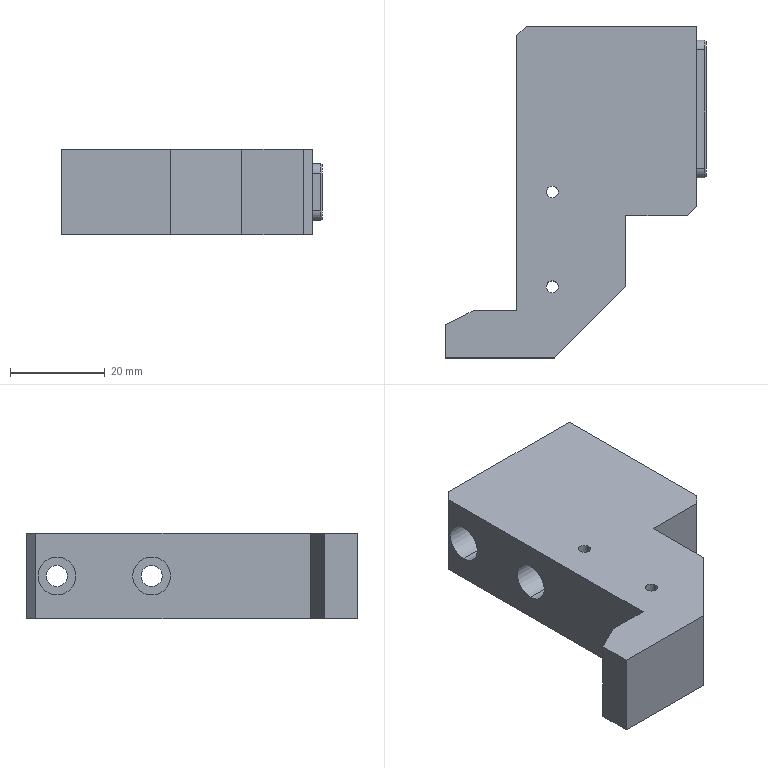Part | NX | features BREP 1 | 1 solid | 45 faces | box 55 x 70 x 18 mm | volume 37396 mm3 | plane 25 | cylinder 16 | cone 4 | commonest cylinder face diameters 2.5 x4 4 x4 4.5 x4 8 x4
STEP:
#1=CARTESIAN_POINT('',(-36.,70.,9.));
#2=VERTEX_POINT('',#1);
#3=CARTESIAN_POINT('',(-38.,68.,9.));
#4=VERTEX_POINT('',#3);
#5=CARTESIAN_POINT('',(-53.,53.,9.));
#6=DIRECTION('',(-0.7071,-0.7071,0.));
#7=VECTOR('',#6,1000.);
#8=LINE('',#5,#7);
#9=EDGE_CURVE('',#2,#4,#8,.T.);
#10=ORIENTED_EDGE('',*,*,#9,.F.);
#11=CARTESIAN_POINT('',(-36.,70.,-9.));
#12=VERTEX_POINT('',#11);
#13=CARTESIAN_POINT('',(-36.,70.,9.));
#14=DIRECTION('',(0.,0.,1.));
#15=VECTOR('',#14,1000.);
#16=LINE('',#13,#15);
#17=EDGE_CURVE('',#12,#2,#16,.T.);
#18=ORIENTED_EDGE('',*,*,#17,.F.);
#19=CARTESIAN_POINT('',(-38.,68.,-9.));
#20=VERTEX_POINT('',#19);
#21=CARTESIAN_POINT('',(-38.,68.,-9.));
#22=DIRECTION('',(0.7071,0.7071,0.));
#23=VECTOR('',#22,1000.);
#24=LINE('',#21,#23);
#25=EDGE_CURVE('',#20,#12,#24,.T.);
#26=ORIENTED_EDGE('',*,*,#25,.F.);
#27=CARTESIAN_POINT('',(-38.,68.,9.));
#28=DIRECTION('',(0.,0.,-1.));
#29=VECTOR('',#28,1000.);
#30=LINE('',#27,#29);
#31=EDGE_CURVE('',#4,#20,#30,.T.);
#32=ORIENTED_EDGE('',*,*,#31,.F.);
#33=EDGE_LOOP('',(#10,#18,#26,#32));
#34=FACE_BOUND('',#33,.T.);
#35=CARTESIAN_POINT('',(-38.,68.,9.));
#36=DIRECTION('',(0.7071,-0.7071,0.));
#37=DIRECTION('',(0.,0.,-1.));
#38=AXIS2_PLACEMENT_3D('',#35,#36,#37);
#39=PLANE('',#38);
#40=ADVANCED_FACE('',(#34),#39,.F.);
#41=CARTESIAN_POINT('',(0.,32.,-9.));
#42=VERTEX_POINT('',#41);
#43=CARTESIAN_POINT('',(-2.,30.,-9.));
#44=VERTEX_POINT('',#43);
#45=CARTESIAN_POINT('',(-2.,30.,-9.));
#46=DIRECTION('',(-0.7071,-0.7071,0.));
#47=VECTOR('',#46,1000.);
#48=LINE('',#45,#47);
#49=EDGE_CURVE('',#42,#44,#48,.T.);
#50=ORIENTED_EDGE('',*,*,#49,.F.);
#51=CARTESIAN_POINT('',(0.,32.,9.));
#52=VERTEX_POINT('',#51);
#53=CARTESIAN_POINT('',(0.,32.,9.));
#54=DIRECTION('',(0.,0.,-1.));
#55=VECTOR('',#54,1000.);
#56=LINE('',#53,#55);
#57=EDGE_CURVE('',#52,#42,#56,.T.);
#58=ORIENTED_EDGE('',*,*,#57,.F.);
#59=CARTESIAN_POINT('',(-2.,30.,9.));
#60=VERTEX_POINT('',#59);
#61=CARTESIAN_POINT('',(-16.,16.,9.));
#62=DIRECTION('',(0.7071,0.7071,0.));
#63=VECTOR('',#62,1000.);
#64=LINE('',#61,#63);
#65=EDGE_CURVE('',#60,#52,#64,.T.);
#66=ORIENTED_EDGE('',*,*,#65,.F.);
#67=CARTESIAN_POINT('',(-2.,30.,-9.));
#68=DIRECTION('',(0.,0.,1.));
#69=VECTOR('',#68,1000.);
#70=LINE('',#67,#69);
#71=EDGE_CURVE('',#44,#60,#70,.T.);
#72=ORIENTED_EDGE('',*,*,#71,.F.);
#73=EDGE_LOOP('',(#50,#58,#66,#72));
#74=FACE_BOUND('',#73,.T.);
#75=CARTESIAN_POINT('',(-2.,30.,-9.));
#76=DIRECTION('',(-0.7071,0.7071,0.));
#77=DIRECTION('',(0.,0.,1.));
#78=AXIS2_PLACEMENT_3D('',#75,#76,#77);
#79=PLANE('',#78);
#80=ADVANCED_FACE('',(#74),#79,.F.);
#81=CARTESIAN_POINT('',(-31.75,35.,9.));
#82=VERTEX_POINT('',#81);
#83=CARTESIAN_POINT('',(-31.75,35.,-9.));
#84=VERTEX_POINT('',#83);
#85=CARTESIAN_POINT('',(-31.75,35.,9.));
#86=DIRECTION('',(0.,0.,1.));
#87=VECTOR('',#86,1000.);
#88=LINE('',#85,#87);
#89=EDGE_CURVE('',#82,#84,#88,.F.);
#90=ORIENTED_EDGE('',*,*,#89,.T.);
#91=CARTESIAN_POINT('',(-29.25,35.,-9.));
#92=VERTEX_POINT('',#91);
#93=CARTESIAN_POINT('',(-30.5,35.,-9.));
#94=DIRECTION('',(0.,0.,1.));
#95=DIRECTION('',(1.,0.,0.));
#96=AXIS2_PLACEMENT_3D('',#93,#94,#95);
#97=CIRCLE('',#96,1.25);
#98=EDGE_CURVE('',#92,#84,#97,.T.);
#99=ORIENTED_EDGE('',*,*,#98,.F.);
#100=CARTESIAN_POINT('',(-29.25,35.,9.));
#101=VERTEX_POINT('',#100);
#102=CARTESIAN_POINT('',(-29.25,35.,9.));
#103=DIRECTION('',(0.,0.,1.));
#104=VECTOR('',#103,1000.);
#105=LINE('',#102,#104);
#106=EDGE_CURVE('',#101,#92,#105,.F.);
#107=ORIENTED_EDGE('',*,*,#106,.F.);
#108=CARTESIAN_POINT('',(-30.5,35.,9.));
#109=DIRECTION('',(0.,0.,1.));
#110=DIRECTION('',(1.,0.,0.));
#111=AXIS2_PLACEMENT_3D('',#108,#109,#110);
#112=CIRCLE('',#111,1.25);
#113=EDGE_CURVE('',#101,#82,#112,.T.);
#114=ORIENTED_EDGE('',*,*,#113,.T.);
#115=EDGE_LOOP('',(#90,#99,#107,#114));
#116=FACE_BOUND('',#115,.T.);
#117=CARTESIAN_POINT('',(-30.5,35.,9.));
#118=DIRECTION('',(0.,0.,1.));
#119=DIRECTION('',(1.,0.,0.));
#120=AXIS2_PLACEMENT_3D('',#117,#118,#119);
#121=CYLINDRICAL_SURFACE('',#120,1.25);
#122=ADVANCED_FACE('',(#116),#121,.F.);
#123=CARTESIAN_POINT('',(-31.75,15.,9.));
#124=VERTEX_POINT('',#123);
#125=CARTESIAN_POINT('',(-31.75,15.,-9.));
#126=VERTEX_POINT('',#125);
#127=CARTESIAN_POINT('',(-31.75,15.,9.));
#128=DIRECTION('',(0.,0.,1.));
#129=VECTOR('',#128,1000.);
#130=LINE('',#127,#129);
#131=EDGE_CURVE('',#124,#126,#130,.F.);
#132=ORIENTED_EDGE('',*,*,#131,.T.);
#133=CARTESIAN_POINT('',(-29.25,15.,-9.));
#134=VERTEX_POINT('',#133);
#135=CARTESIAN_POINT('',(-30.5,15.,-9.));
#136=DIRECTION('',(0.,0.,1.));
#137=DIRECTION('',(1.,0.,0.));
#138=AXIS2_PLACEMENT_3D('',#135,#136,#137);
#139=CIRCLE('',#138,1.25);
#140=EDGE_CURVE('',#134,#126,#139,.T.);
#141=ORIENTED_EDGE('',*,*,#140,.F.);
#142=CARTESIAN_POINT('',(-29.25,15.,9.));
#143=VERTEX_POINT('',#142);
#144=CARTESIAN_POINT('',(-29.25,15.,9.));
#145=DIRECTION('',(0.,0.,1.));
#146=VECTOR('',#145,1000.);
#147=LINE('',#144,#146);
#148=EDGE_CURVE('',#143,#134,#147,.F.);
#149=ORIENTED_EDGE('',*,*,#148,.F.);
#150=CARTESIAN_POINT('',(-30.5,15.,9.));
#151=DIRECTION('',(0.,0.,1.));
#152=DIRECTION('',(1.,0.,0.));
#153=AXIS2_PLACEMENT_3D('',#150,#151,#152);
#154=CIRCLE('',#153,1.25);
#155=EDGE_CURVE('',#143,#124,#154,.T.);
#156=ORIENTED_EDGE('',*,*,#155,.T.);
#157=EDGE_LOOP('',(#132,#141,#149,#156));
#158=FACE_BOUND('',#157,.T.);
#159=CARTESIAN_POINT('',(-30.5,15.,9.));
#160=DIRECTION('',(0.,0.,1.));
#161=DIRECTION('',(1.,0.,0.));
#162=AXIS2_PLACEMENT_3D('',#159,#160,#161);
#163=CYLINDRICAL_SURFACE('',#162,1.25);
#164=ADVANCED_FACE('',(#158),#163,.F.);
#165=CARTESIAN_POINT('',(-30.,0.,9.));
#166=VERTEX_POINT('',#165);
#167=CARTESIAN_POINT('',(-15.,15.,9.));
#168=VERTEX_POINT('',#167);
#169=CARTESIAN_POINT('',(-15.,15.,9.));
#170=DIRECTION('',(0.7071,0.7071,0.));
#171=VECTOR('',#170,1000.);
#172=LINE('',#169,#171);
#173=EDGE_CURVE('',#166,#168,#172,.T.);
#174=ORIENTED_EDGE('',*,*,#173,.F.);
#175=CARTESIAN_POINT('',(-30.,0.,-9.));
#176=VERTEX_POINT('',#175);
#177=CARTESIAN_POINT('',(-30.,0.,9.));
#178=DIRECTION('',(0.,0.,1.));
#179=VECTOR('',#178,1000.);
#180=LINE('',#177,#179);
#181=EDGE_CURVE('',#176,#166,#180,.T.);
#182=ORIENTED_EDGE('',*,*,#181,.F.);
#183=CARTESIAN_POINT('',(-15.,15.,-9.));
#184=VERTEX_POINT('',#183);
#185=CARTESIAN_POINT('',(-15.,15.,-9.));
#186=DIRECTION('',(-0.7071,-0.7071,0.));
#187=VECTOR('',#186,1000.);
#188=LINE('',#185,#187);
#189=EDGE_CURVE('',#184,#176,#188,.T.);
#190=ORIENTED_EDGE('',*,*,#189,.F.);
#191=CARTESIAN_POINT('',(-15.,15.,-9.));
#192=DIRECTION('',(0.,0.,-1.));
#193=VECTOR('',#192,1000.);
#194=LINE('',#191,#193);
#195=EDGE_CURVE('',#168,#184,#194,.T.);
#196=ORIENTED_EDGE('',*,*,#195,.F.);
#197=EDGE_LOOP('',(#174,#182,#190,#196));
#198=FACE_BOUND('',#197,.T.);
#199=CARTESIAN_POINT('',(-15.,15.,0.));
#200=DIRECTION('',(0.7071,-0.7071,0.));
#201=DIRECTION('',(0.,0.,1.));
#202=AXIS2_PLACEMENT_3D('',#199,#200,#201);
#203=PLANE('',#202);
#204=ADVANCED_FACE('',(#198),#203,.T.);
#205=CARTESIAN_POINT('',(2.,65.,5.7));
#206=VERTEX_POINT('',#205);
#207=CARTESIAN_POINT('',(1.7,65.,6.));
#208=VERTEX_POINT('',#207);
#209=CARTESIAN_POINT('',(2.,65.,5.7));
#210=DIRECTION('',(-0.7071,0.,0.7071));
#211=VECTOR('',#210,1000.);
#212=LINE('',#209,#211);
#213=EDGE_CURVE('',#206,#208,#212,.T.);
#214=ORIENTED_EDGE('',*,*,#213,.T.);
#215=CARTESIAN_POINT('',(1.7,40.,6.));
#216=VERTEX_POINT('',#215);
#217=CARTESIAN_POINT('',(1.7,38.,6.));
#218=DIRECTION('',(0.,1.,0.));
#219=VECTOR('',#218,1000.);
#220=LINE('',#217,#219);
#221=EDGE_CURVE('',#216,#208,#220,.T.);
#222=ORIENTED_EDGE('',*,*,#221,.F.);
#223=CARTESIAN_POINT('',(2.,40.,5.7));
#224=VERTEX_POINT('',#223);
#225=CARTESIAN_POINT('',(1.7,40.,6.));
#226=DIRECTION('',(0.7071,0.,-0.7071));
#227=VECTOR('',#226,1000.);
#228=LINE('',#225,#227);
#229=EDGE_CURVE('',#216,#224,#228,.T.);
#230=ORIENTED_EDGE('',*,*,#229,.T.);
#231=CARTESIAN_POINT('',(2.,0.,5.7));
#232=DIRECTION('',(0.,-1.,0.));
#233=VECTOR('',#232,1000.);
#234=LINE('',#231,#233);
#235=EDGE_CURVE('',#206,#224,#234,.T.);
#236=ORIENTED_EDGE('',*,*,#235,.F.);
#237=EDGE_LOOP('',(#214,#222,#230,#236));
#238=FACE_BOUND('',#237,.T.);
#239=CARTESIAN_POINT('',(2.,0.,5.7));
#240=DIRECTION('',(-0.7071,0.,-0.7071));
#241=DIRECTION('',(0.,-1.,0.));
#242=AXIS2_PLACEMENT_3D('',#239,#240,#241);
#243=PLANE('',#242);
#244=ADVANCED_FACE('',(#238),#243,.F.);
#245=CARTESIAN_POINT('',(1.7,38.,4.));
#246=VERTEX_POINT('',#245);
#247=CARTESIAN_POINT('',(2.,38.3,4.));
#248=VERTEX_POINT('',#247);
#249=CARTESIAN_POINT('',(1.7,38.,4.));
#250=DIRECTION('',(0.7071,0.7071,0.));
#251=VECTOR('',#250,1000.);
#252=LINE('',#249,#251);
#253=EDGE_CURVE('',#246,#248,#252,.T.);
#254=ORIENTED_EDGE('',*,*,#253,.T.);
#255=CARTESIAN_POINT('',(2.,40.,4.));
#256=DIRECTION('',(1.,0.,0.));
#257=DIRECTION('',(0.,0.,1.));
#258=AXIS2_PLACEMENT_3D('',#255,#256,#257);
#259=CIRCLE('',#258,1.7);
#260=EDGE_CURVE('',#224,#248,#259,.T.);
#261=ORIENTED_EDGE('',*,*,#260,.F.);
#262=ORIENTED_EDGE('',*,*,#229,.F.);
#263=CARTESIAN_POINT('',(1.7,40.,4.));
#264=DIRECTION('',(-1.,0.,0.));
#265=DIRECTION('',(0.,0.,1.));
#266=AXIS2_PLACEMENT_3D('',#263,#264,#265);
#267=CIRCLE('',#266,2.);
#268=EDGE_CURVE('',#246,#216,#267,.T.);
#269=ORIENTED_EDGE('',*,*,#268,.F.);
#270=EDGE_LOOP('',(#254,#261,#262,#269));
#271=FACE_BOUND('',#270,.T.);
#272=CARTESIAN_POINT('',(2.,40.,4.));
#273=DIRECTION('',(-1.,0.,0.));
#274=DIRECTION('',(0.,0.,1.));
#275=AXIS2_PLACEMENT_3D('',#272,#273,#274);
#276=CONICAL_SURFACE('',#275,1.7,0.7854);
#277=ADVANCED_FACE('',(#271),#276,.T.);
#278=CARTESIAN_POINT('',(2.,66.7,4.));
#279=VERTEX_POINT('',#278);
#280=CARTESIAN_POINT('',(1.7,67.,4.));
#281=VERTEX_POINT('',#280);
#282=CARTESIAN_POINT('',(2.,66.7,4.));
#283=DIRECTION('',(-0.7071,0.7071,0.));
#284=VECTOR('',#283,1000.);
#285=LINE('',#282,#284);
#286=EDGE_CURVE('',#279,#281,#285,.T.);
#287=ORIENTED_EDGE('',*,*,#286,.T.);
#288=CARTESIAN_POINT('',(1.7,65.,4.));
#289=DIRECTION('',(-1.,0.,0.));
#290=DIRECTION('',(0.,0.,1.));
#291=AXIS2_PLACEMENT_3D('',#288,#289,#290);
#292=CIRCLE('',#291,2.);
#293=EDGE_CURVE('',#208,#281,#292,.T.);
#294=ORIENTED_EDGE('',*,*,#293,.F.);
#295=ORIENTED_EDGE('',*,*,#213,.F.);
#296=CARTESIAN_POINT('',(2.,65.,4.));
#297=DIRECTION('',(1.,0.,0.));
#298=DIRECTION('',(0.,0.,1.));
#299=AXIS2_PLACEMENT_3D('',#296,#297,#298);
#300=CIRCLE('',#299,1.7);
#301=EDGE_CURVE('',#279,#206,#300,.T.);
#302=ORIENTED_EDGE('',*,*,#301,.F.);
#303=EDGE_LOOP('',(#287,#294,#295,#302));
#304=FACE_BOUND('',#303,.T.);
#305=CARTESIAN_POINT('',(2.,65.,4.));
#306=DIRECTION('',(-1.,0.,0.));
#307=DIRECTION('',(0.,0.,1.));
#308=AXIS2_PLACEMENT_3D('',#305,#306,#307);
#309=CONICAL_SURFACE('',#308,1.7,0.7854);
#310=ADVANCED_FACE('',(#304),#309,.T.);
#311=CARTESIAN_POINT('',(1.7,38.,-4.));
#312=VERTEX_POINT('',#311);
#313=CARTESIAN_POINT('',(2.,38.3,-4.));
#314=VERTEX_POINT('',#313);
#315=CARTESIAN_POINT('',(1.7,38.,-4.));
#316=DIRECTION('',(0.7071,0.7071,0.));
#317=VECTOR('',#316,1000.);
#318=LINE('',#315,#317);
#319=EDGE_CURVE('',#312,#314,#318,.T.);
#320=ORIENTED_EDGE('',*,*,#319,.T.);
#321=CARTESIAN_POINT('',(2.,38.3,0.));
#322=DIRECTION('',(0.,0.,-1.));
#323=VECTOR('',#322,1000.);
#324=LINE('',#321,#323);
#325=EDGE_CURVE('',#248,#314,#324,.T.);
#326=ORIENTED_EDGE('',*,*,#325,.F.);
#327=ORIENTED_EDGE('',*,*,#253,.F.);
#328=CARTESIAN_POINT('',(1.7,38.,6.));
#329=DIRECTION('',(0.,0.,1.));
#330=VECTOR('',#329,1000.);
#331=LINE('',#328,#330);
#332=EDGE_CURVE('',#312,#246,#331,.T.);
#333=ORIENTED_EDGE('',*,*,#332,.F.);
#334=EDGE_LOOP('',(#320,#326,#327,#333));
#335=FACE_BOUND('',#334,.T.);
#336=CARTESIAN_POINT('',(2.,38.3,0.));
#337=DIRECTION('',(-0.7071,0.7071,0.));
#338=DIRECTION('',(0.,0.,-1.));
#339=AXIS2_PLACEMENT_3D('',#336,#337,#338);
#340=PLANE('',#339);
#341=ADVANCED_FACE('',(#335),#340,.F.);
#342=CARTESIAN_POINT('',(2.,66.7,-4.));
#343=VERTEX_POINT('',#342);
#344=CARTESIAN_POINT('',(1.7,67.,-4.));
#345=VERTEX_POINT('',#344);
#346=CARTESIAN_POINT('',(2.,66.7,-4.));
#347=DIRECTION('',(-0.7071,0.7071,0.));
#348=VECTOR('',#347,1000.);
#349=LINE('',#346,#348);
#350=EDGE_CURVE('',#343,#345,#349,.T.);
#351=ORIENTED_EDGE('',*,*,#350,.T.);
#352=CARTESIAN_POINT('',(1.7,67.,6.));
#353=DIRECTION('',(0.,0.,-1.));
#354=VECTOR('',#353,1000.);
#355=LINE('',#352,#354);
#356=EDGE_CURVE('',#281,#345,#355,.T.);
#357=ORIENTED_EDGE('',*,*,#356,.F.);
#358=ORIENTED_EDGE('',*,*,#286,.F.);
#359=CARTESIAN_POINT('',(2.,66.7,0.));
#360=DIRECTION('',(0.,0.,1.));
#361=VECTOR('',#360,1000.);
#362=LINE('',#359,#361);
#363=EDGE_CURVE('',#343,#279,#362,.T.);
#364=ORIENTED_EDGE('',*,*,#363,.F.);
#365=EDGE_LOOP('',(#351,#357,#358,#364));
#366=FACE_BOUND('',#365,.T.);
#367=CARTESIAN_POINT('',(2.,66.7,0.));
#368=DIRECTION('',(-0.7071,-0.7071,0.));
#369=DIRECTION('',(0.,0.,1.));
#370=AXIS2_PLACEMENT_3D('',#367,#368,#369);
#371=PLANE('',#370);
#372=ADVANCED_FACE('',(#366),#371,.F.);
#373=CARTESIAN_POINT('',(1.7,40.,-6.));
#374=VERTEX_POINT('',#373);
#375=CARTESIAN_POINT('',(2.,40.,-5.7));
#376=VERTEX_POINT('',#375);
#377=CARTESIAN_POINT('',(1.7,40.,-6.));
#378=DIRECTION('',(0.7071,0.,0.7071));
#379=VECTOR('',#378,1000.);
#380=LINE('',#377,#379);
#381=EDGE_CURVE('',#374,#376,#380,.T.);
#382=ORIENTED_EDGE('',*,*,#381,.T.);
#383=CARTESIAN_POINT('',(2.,40.,-4.));
#384=DIRECTION('',(1.,0.,0.));
#385=DIRECTION('',(0.,0.,1.));
#386=AXIS2_PLACEMENT_3D('',#383,#384,#385);
#387=CIRCLE('',#386,1.7);
#388=EDGE_CURVE('',#314,#376,#387,.T.);
#389=ORIENTED_EDGE('',*,*,#388,.F.);
#390=ORIENTED_EDGE('',*,*,#319,.F.);
#391=CARTESIAN_POINT('',(1.7,40.,-4.));
#392=DIRECTION('',(-1.,0.,0.));
#393=DIRECTION('',(0.,0.,1.));
#394=AXIS2_PLACEMENT_3D('',#391,#392,#393);
#395=CIRCLE('',#394,2.);
#396=EDGE_CURVE('',#374,#312,#395,.T.);
#397=ORIENTED_EDGE('',*,*,#396,.F.);
#398=EDGE_LOOP('',(#382,#389,#390,#397));
#399=FACE_BOUND('',#398,.T.);
#400=CARTESIAN_POINT('',(2.,40.,-4.));
#401=DIRECTION('',(-1.,0.,0.));
#402=DIRECTION('',(0.,0.,1.));
#403=AXIS2_PLACEMENT_3D('',#400,#401,#402);
#404=CONICAL_SURFACE('',#403,1.7,0.7854);
#405=ADVANCED_FACE('',(#399),#404,.T.);
#406=CARTESIAN_POINT('',(2.,65.,-5.7));
#407=VERTEX_POINT('',#406);
#408=CARTESIAN_POINT('',(1.7,65.,-6.));
#409=VERTEX_POINT('',#408);
#410=CARTESIAN_POINT('',(2.,65.,-5.7));
#411=DIRECTION('',(-0.7071,0.,-0.7071));
#412=VECTOR('',#411,1000.);
#413=LINE('',#410,#412);
#414=EDGE_CURVE('',#407,#409,#413,.T.);
#415=ORIENTED_EDGE('',*,*,#414,.T.);
#416=CARTESIAN_POINT('',(1.7,65.,-4.));
#417=DIRECTION('',(-1.,0.,0.));
#418=DIRECTION('',(0.,0.,1.));
#419=AXIS2_PLACEMENT_3D('',#416,#417,#418);
#420=CIRCLE('',#419,2.);
#421=EDGE_CURVE('',#345,#409,#420,.T.);
#422=ORIENTED_EDGE('',*,*,#421,.F.);
#423=ORIENTED_EDGE('',*,*,#350,.F.);
#424=CARTESIAN_POINT('',(2.,65.,-4.));
#425=DIRECTION('',(1.,0.,0.));
#426=DIRECTION('',(0.,0.,1.));
#427=AXIS2_PLACEMENT_3D('',#424,#425,#426);
#428=CIRCLE('',#427,1.7);
#429=EDGE_CURVE('',#407,#343,#428,.T.);
#430=ORIENTED_EDGE('',*,*,#429,.F.);
#431=EDGE_LOOP('',(#415,#422,#423,#430));
#432=FACE_BOUND('',#431,.T.);
#433=CARTESIAN_POINT('',(2.,65.,-4.));
#434=DIRECTION('',(-1.,0.,0.));
#435=DIRECTION('',(0.,0.,1.));
#436=AXIS2_PLACEMENT_3D('',#433,#434,#435);
#437=CONICAL_SURFACE('',#436,1.7,0.7854);
#438=ADVANCED_FACE('',(#432),#437,.T.);
#439=ORIENTED_EDGE('',*,*,#381,.F.);
#440=CARTESIAN_POINT('',(1.7,38.,-6.));
#441=DIRECTION('',(0.,-1.,0.));
#442=VECTOR('',#441,1000.);
#443=LINE('',#440,#442);
#444=EDGE_CURVE('',#409,#374,#443,.T.);
#445=ORIENTED_EDGE('',*,*,#444,.F.);
#446=ORIENTED_EDGE('',*,*,#414,.F.);
#447=CARTESIAN_POINT('',(2.,0.,-5.7));
#448=DIRECTION('',(0.,1.,0.));
#449=VECTOR('',#448,1000.);
#450=LINE('',#447,#449);
#451=EDGE_CURVE('',#376,#407,#450,.T.);
#452=ORIENTED_EDGE('',*,*,#451,.F.);
#453=EDGE_LOOP('',(#439,#445,#446,#452));
#454=FACE_BOUND('',#453,.T.);
#455=CARTESIAN_POINT('',(2.,0.,-5.7));
#456=DIRECTION('',(-0.7071,0.,0.7071));
#457=DIRECTION('',(0.,1.,0.));
#458=AXIS2_PLACEMENT_3D('',#455,#456,#457);
#459=PLANE('',#458);
#460=ADVANCED_FACE('',(#454),#459,.F.);
#461=CARTESIAN_POINT('',(0.,67.,-4.));
#462=VERTEX_POINT('',#461);
#463=CARTESIAN_POINT('',(2.,67.,-4.));
#464=DIRECTION('',(-1.,0.,0.));
#465=VECTOR('',#464,1000.);
#466=LINE('',#463,#465);
#467=EDGE_CURVE('',#345,#462,#466,.T.);
#468=ORIENTED_EDGE('',*,*,#467,.F.);
#469=ORIENTED_EDGE('',*,*,#421,.T.);
#470=CARTESIAN_POINT('',(0.,65.,-6.));
#471=VERTEX_POINT('',#470);
#472=CARTESIAN_POINT('',(2.,65.,-6.));
#473=DIRECTION('',(1.,0.,0.));
#474=VECTOR('',#473,1000.);
#475=LINE('',#472,#474);
#476=EDGE_CURVE('',#471,#409,#475,.T.);
#477=ORIENTED_EDGE('',*,*,#476,.F.);
#478=CARTESIAN_POINT('',(0.,65.,-4.));
#479=DIRECTION('',(-1.,0.,0.));
#480=DIRECTION('',(0.,0.,1.));
#481=AXIS2_PLACEMENT_3D('',#478,#479,#480);
#482=CIRCLE('',#481,2.);
#483=EDGE_CURVE('',#462,#471,#482,.T.);
#484=ORIENTED_EDGE('',*,*,#483,.F.);
#485=EDGE_LOOP('',(#468,#469,#477,#484));
#486=FACE_BOUND('',#485,.T.);
#487=CARTESIAN_POINT('',(2.,65.,-4.));
#488=DIRECTION('',(-1.,0.,0.));
#489=DIRECTION('',(0.,0.,1.));
#490=AXIS2_PLACEMENT_3D('',#487,#488,#489);
#491=CYLINDRICAL_SURFACE('',#490,2.);
#492=ADVANCED_FACE('',(#486),#491,.T.);
#493=CARTESIAN_POINT('',(0.,65.,6.));
#494=VERTEX_POINT('',#493);
#495=CARTESIAN_POINT('',(2.,65.,6.));
#496=DIRECTION('',(-1.,0.,0.));
#497=VECTOR('',#496,1000.);
#498=LINE('',#495,#497);
#499=EDGE_CURVE('',#208,#494,#498,.T.);
#500=ORIENTED_EDGE('',*,*,#499,.F.);
#501=ORIENTED_EDGE('',*,*,#293,.T.);
#502=CARTESIAN_POINT('',(0.,67.,4.));
#503=VERTEX_POINT('',#502);
#504=CARTESIAN_POINT('',(2.,67.,4.));
#505=DIRECTION('',(1.,0.,0.));
#506=VECTOR('',#505,1000.);
#507=LINE('',#504,#506);
#508=EDGE_CURVE('',#503,#281,#507,.T.);
#509=ORIENTED_EDGE('',*,*,#508,.F.);
#510=CARTESIAN_POINT('',(0.,65.,4.));
#511=DIRECTION('',(-1.,0.,0.));
#512=DIRECTION('',(0.,0.,1.));
#513=AXIS2_PLACEMENT_3D('',#510,#511,#512);
#514=CIRCLE('',#513,2.);
#515=EDGE_CURVE('',#494,#503,#514,.T.);
#516=ORIENTED_EDGE('',*,*,#515,.F.);
#517=EDGE_LOOP('',(#500,#501,#509,#516));
#518=FACE_BOUND('',#517,.T.);
#519=CARTESIAN_POINT('',(2.,65.,4.));
#520=DIRECTION('',(-1.,0.,0.));
#521=DIRECTION('',(0.,0.,1.));
#522=AXIS2_PLACEMENT_3D('',#519,#520,#521);
#523=CYLINDRICAL_SURFACE('',#522,2.);
#524=ADVANCED_FACE('',(#518),#523,.T.);
#525=CARTESIAN_POINT('',(0.,40.,-6.));
#526=VERTEX_POINT('',#525);
#527=CARTESIAN_POINT('',(2.,40.,-6.));
#528=DIRECTION('',(-1.,0.,0.));
#529=VECTOR('',#528,1000.);
#530=LINE('',#527,#529);
#531=EDGE_CURVE('',#374,#526,#530,.T.);
#532=ORIENTED_EDGE('',*,*,#531,.F.);
#533=ORIENTED_EDGE('',*,*,#396,.T.);
#534=CARTESIAN_POINT('',(0.,38.,-4.));
#535=VERTEX_POINT('',#534);
#536=CARTESIAN_POINT('',(2.,38.,-4.));
#537=DIRECTION('',(1.,0.,0.));
#538=VECTOR('',#537,1000.);
#539=LINE('',#536,#538);
#540=EDGE_CURVE('',#535,#312,#539,.T.);
#541=ORIENTED_EDGE('',*,*,#540,.F.);
#542=CARTESIAN_POINT('',(0.,40.,-4.));
#543=DIRECTION('',(-1.,0.,0.));
#544=DIRECTION('',(0.,0.,1.));
#545=AXIS2_PLACEMENT_3D('',#542,#543,#544);
#546=CIRCLE('',#545,2.);
#547=EDGE_CURVE('',#526,#535,#546,.T.);
#548=ORIENTED_EDGE('',*,*,#547,.F.);
#549=EDGE_LOOP('',(#532,#533,#541,#548));
#550=FACE_BOUND('',#549,.T.);
#551=CARTESIAN_POINT('',(2.,40.,-4.));
#552=DIRECTION('',(-1.,0.,0.));
#553=DIRECTION('',(0.,0.,1.));
#554=AXIS2_PLACEMENT_3D('',#551,#552,#553);
#555=CYLINDRICAL_SURFACE('',#554,2.);
#556=ADVANCED_FACE('',(#550),#555,.T.);
#557=CARTESIAN_POINT('',(0.,38.,4.));
#558=VERTEX_POINT('',#557);
#559=CARTESIAN_POINT('',(2.,38.,4.));
#560=DIRECTION('',(-1.,0.,0.));
#561=VECTOR('',#560,1000.);
#562=LINE('',#559,#561);
#563=EDGE_CURVE('',#246,#558,#562,.T.);
#564=ORIENTED_EDGE('',*,*,#563,.F.);
#565=ORIENTED_EDGE('',*,*,#268,.T.);
#566=CARTESIAN_POINT('',(0.,40.,6.));
#567=VERTEX_POINT('',#566);
#568=CARTESIAN_POINT('',(2.,40.,6.));
#569=DIRECTION('',(1.,0.,0.));
#570=VECTOR('',#569,1000.);
#571=LINE('',#568,#570);
#572=EDGE_CURVE('',#567,#216,#571,.T.);
#573=ORIENTED_EDGE('',*,*,#572,.F.);
#574=CARTESIAN_POINT('',(0.,40.,4.));
#575=DIRECTION('',(-1.,0.,0.));
#576=DIRECTION('',(0.,0.,1.));
#577=AXIS2_PLACEMENT_3D('',#574,#575,#576);
#578=CIRCLE('',#577,2.);
#579=EDGE_CURVE('',#558,#567,#578,.T.);
#580=ORIENTED_EDGE('',*,*,#579,.F.);
#581=EDGE_LOOP('',(#564,#565,#573,#580));
#582=FACE_BOUND('',#581,.T.);
#583=CARTESIAN_POINT('',(2.,40.,4.));
#584=DIRECTION('',(-1.,0.,0.));
#585=DIRECTION('',(0.,0.,1.));
#586=AXIS2_PLACEMENT_3D('',#583,#584,#585);
#587=CYLINDRICAL_SURFACE('',#586,2.);
#588=ADVANCED_FACE('',(#582),#587,.T.);
#589=CARTESIAN_POINT('',(-15.,30.,9.));
#590=VERTEX_POINT('',#589);
#591=CARTESIAN_POINT('',(-15.,0.,9.));
#592=DIRECTION('',(0.,-1.,0.));
#593=VECTOR('',#592,1000.);
#594=LINE('',#591,#593);
#595=EDGE_CURVE('',#590,#168,#594,.T.);
#596=ORIENTED_EDGE('',*,*,#595,.T.);
#597=ORIENTED_EDGE('',*,*,#195,.T.);
#598=CARTESIAN_POINT('',(-15.,30.,-9.));
#599=VERTEX_POINT('',#598);
#600=CARTESIAN_POINT('',(-15.,0.,-9.));
#601=DIRECTION('',(0.,1.,0.));
#602=VECTOR('',#601,1000.);
#603=LINE('',#600,#602);
#604=EDGE_CURVE('',#184,#599,#603,.T.);
#605=ORIENTED_EDGE('',*,*,#604,.T.);
#606=CARTESIAN_POINT('',(-15.,30.,-9.));
#607=DIRECTION('',(0.,0.,1.));
#608=VECTOR('',#607,1000.);
#609=LINE('',#606,#608);
#610=EDGE_CURVE('',#599,#590,#609,.T.);
#611=ORIENTED_EDGE('',*,*,#610,.T.);
#612=EDGE_LOOP('',(#596,#597,#605,#611));
#613=FACE_BOUND('',#612,.T.);
#614=CARTESIAN_POINT('',(-15.,0.,0.));
#615=DIRECTION('',(1.,0.,0.));
#616=DIRECTION('',(0.,0.,-1.));
#617=AXIS2_PLACEMENT_3D('',#614,#615,#616);
#618=PLANE('',#617);
#619=ADVANCED_FACE('',(#613),#618,.T.);
#620=CARTESIAN_POINT('',(-15.,30.,-9.));
#621=DIRECTION('',(1.,0.,0.));
#622=VECTOR('',#621,1000.);
#623=LINE('',#620,#622);
#624=EDGE_CURVE('',#599,#44,#623,.T.);
#625=ORIENTED_EDGE('',*,*,#624,.T.);
#626=ORIENTED_EDGE('',*,*,#71,.T.);
#627=CARTESIAN_POINT('',(-15.,30.,9.));
#628=DIRECTION('',(1.,0.,0.));
#629=VECTOR('',#628,1000.);
#630=LINE('',#627,#629);
#631=EDGE_CURVE('',#590,#60,#630,.T.);
#632=ORIENTED_EDGE('',*,*,#631,.F.);
#633=ORIENTED_EDGE('',*,*,#610,.F.);
#634=EDGE_LOOP('',(#625,#626,#632,#633));
#635=FACE_BOUND('',#634,.T.);
#636=CARTESIAN_POINT('',(-15.,30.,-9.));
#637=DIRECTION('',(0.,1.,0.));
#638=DIRECTION('',(0.,0.,1.));
#639=AXIS2_PLACEMENT_3D('',#636,#637,#638);
#640=PLANE('',#639);
#641=ADVANCED_FACE('',(#635),#640,.F.);
#642=CARTESIAN_POINT('',(-47.,10.,9.));
#643=VERTEX_POINT('',#642);
#644=CARTESIAN_POINT('',(-53.,7.,9.));
#645=VERTEX_POINT('',#644);
#646=CARTESIAN_POINT('',(-13.4,26.8,9.));
#647=DIRECTION('',(-0.8944,-0.4472,0.));
#648=VECTOR('',#647,1000.);
#649=LINE('',#646,#648);
#650=EDGE_CURVE('',#643,#645,#649,.T.);
#651=ORIENTED_EDGE('',*,*,#650,.F.);
#652=CARTESIAN_POINT('',(-47.,10.,-9.));
#653=VERTEX_POINT('',#652);
#654=CARTESIAN_POINT('',(-47.,10.,9.));
#655=DIRECTION('',(0.,0.,1.));
#656=VECTOR('',#655,1000.);
#657=LINE('',#654,#656);
#658=EDGE_CURVE('',#653,#643,#657,.T.);
#659=ORIENTED_EDGE('',*,*,#658,.F.);
#660=CARTESIAN_POINT('',(-53.,7.,-9.));
#661=VERTEX_POINT('',#660);
#662=CARTESIAN_POINT('',(-53.,7.,-9.));
#663=DIRECTION('',(0.8944,0.4472,0.));
#664=VECTOR('',#663,1000.);
#665=LINE('',#662,#664);
#666=EDGE_CURVE('',#661,#653,#665,.T.);
#667=ORIENTED_EDGE('',*,*,#666,.F.);
#668=CARTESIAN_POINT('',(-53.,7.,9.));
#669=DIRECTION('',(0.,0.,-1.));
#670=VECTOR('',#669,1000.);
#671=LINE('',#668,#670);
#672=EDGE_CURVE('',#645,#661,#671,.T.);
#673=ORIENTED_EDGE('',*,*,#672,.F.);
#674=EDGE_LOOP('',(#651,#659,#667,#673));
#675=FACE_BOUND('',#674,.T.);
#676=CARTESIAN_POINT('',(-53.,7.,9.));
#677=DIRECTION('',(0.4472,-0.8944,0.));
#678=DIRECTION('',(0.,0.,-1.));
#679=AXIS2_PLACEMENT_3D('',#676,#677,#678);
#680=PLANE('',#679);
#681=ADVANCED_FACE('',(#675),#680,.F.);
#682=CARTESIAN_POINT('',(-38.,63.5,-4.));
#683=VERTEX_POINT('',#682);
#684=CARTESIAN_POINT('',(-8.,63.5,-4.));
#685=VERTEX_POINT('',#684);
#686=CARTESIAN_POINT('',(-38.,63.5,-4.));
#687=DIRECTION('',(-1.,0.,0.));
#688=VECTOR('',#687,1000.);
#689=LINE('',#686,#688);
#690=EDGE_CURVE('',#683,#685,#689,.F.);
#691=ORIENTED_EDGE('',*,*,#690,.T.);
#692=CARTESIAN_POINT('',(-8.,63.5,4.));
#693=VERTEX_POINT('',#692);
#694=CARTESIAN_POINT('',(-8.,63.5,0.));
#695=DIRECTION('',(-1.,0.,0.));
#696=DIRECTION('',(0.,0.,1.));
#697=AXIS2_PLACEMENT_3D('',#694,#695,#696);
#698=CIRCLE('',#697,4.);
#699=EDGE_CURVE('',#693,#685,#698,.T.);
#700=ORIENTED_EDGE('',*,*,#699,.F.);
#701=CARTESIAN_POINT('',(-38.,63.5,4.));
#702=VERTEX_POINT('',#701);
#703=CARTESIAN_POINT('',(-38.,63.5,4.));
#704=DIRECTION('',(-1.,0.,0.));
#705=VECTOR('',#704,1000.);
#706=LINE('',#703,#705);
#707=EDGE_CURVE('',#702,#693,#706,.F.);
#708=ORIENTED_EDGE('',*,*,#707,.F.);
#709=CARTESIAN_POINT('',(-38.,63.5,0.));
#710=DIRECTION('',(-1.,0.,0.));
#711=DIRECTION('',(0.,0.,1.));
#712=AXIS2_PLACEMENT_3D('',#709,#710,#711);
#713=CIRCLE('',#712,4.);
#714=EDGE_CURVE('',#702,#683,#713,.T.);
#715=ORIENTED_EDGE('',*,*,#714,.T.);
#716=EDGE_LOOP('',(#691,#700,#708,#715));
#717=FACE_BOUND('',#716,.T.);
#718=CARTESIAN_POINT('',(-38.,63.5,0.));
#719=DIRECTION('',(-1.,0.,0.));
#720=DIRECTION('',(0.,0.,1.));
#721=AXIS2_PLACEMENT_3D('',#718,#719,#720);
#722=CYLINDRICAL_SURFACE('',#721,4.);
#723=ADVANCED_FACE('',(#717),#722,.F.);
#724=ORIENTED_EDGE('',*,*,#699,.T.);
#725=CARTESIAN_POINT('',(-8.,63.5,0.));
#726=DIRECTION('',(-1.,0.,0.));
#727=DIRECTION('',(0.,0.,1.));
#728=AXIS2_PLACEMENT_3D('',#725,#726,#727);
#729=CIRCLE('',#728,4.);
#730=EDGE_CURVE('',#685,#693,#729,.T.);
#731=ORIENTED_EDGE('',*,*,#730,.T.);
#732=EDGE_LOOP('',(#724,#731));
#733=FACE_BOUND('',#732,.T.);
#734=CARTESIAN_POINT('',(-8.,63.5,2.25));
#735=VERTEX_POINT('',#734);
#736=CARTESIAN_POINT('',(-8.,63.5,-2.25));
#737=VERTEX_POINT('',#736);
#738=CARTESIAN_POINT('',(-8.,63.5,0.));
#739=DIRECTION('',(-1.,0.,0.));
#740=DIRECTION('',(0.,0.,1.));
#741=AXIS2_PLACEMENT_3D('',#738,#739,#740);
#742=CIRCLE('',#741,2.25);
#743=EDGE_CURVE('',#735,#737,#742,.T.);
#744=ORIENTED_EDGE('',*,*,#743,.F.);
#745=CARTESIAN_POINT('',(-8.,63.5,0.));
#746=DIRECTION('',(-1.,0.,0.));
#747=DIRECTION('',(0.,0.,1.));
#748=AXIS2_PLACEMENT_3D('',#745,#746,#747);
#749=CIRCLE('',#748,2.25);
#750=EDGE_CURVE('',#737,#735,#749,.T.);
#751=ORIENTED_EDGE('',*,*,#750,.F.);
#752=EDGE_LOOP('',(#744,#751));
#753=FACE_BOUND('',#752,.T.);
#754=CARTESIAN_POINT('',(-8.,65.75,0.));
#755=DIRECTION('',(1.,0.,0.));
#756=DIRECTION('',(0.,0.,-1.));
#757=AXIS2_PLACEMENT_3D('',#754,#755,#756);
#758=PLANE('',#757);
#759=ADVANCED_FACE('',(#733,#753),#758,.F.);
#760=CARTESIAN_POINT('',(2.,63.5,-2.25));
#761=VERTEX_POINT('',#760);
#762=CARTESIAN_POINT('',(-38.,63.5,-2.25));
#763=DIRECTION('',(-1.,0.,0.));
#764=VECTOR('',#763,1000.);
#765=LINE('',#762,#764);
#766=EDGE_CURVE('',#737,#761,#765,.F.);
#767=ORIENTED_EDGE('',*,*,#766,.T.);
#768=CARTESIAN_POINT('',(2.,63.5,2.25));
#769=VERTEX_POINT('',#768);
#770=CARTESIAN_POINT('',(2.,63.5,0.));
#771=DIRECTION('',(-1.,0.,0.));
#772=DIRECTION('',(0.,0.,1.));
#773=AXIS2_PLACEMENT_3D('',#770,#771,#772);
#774=CIRCLE('',#773,2.25);
#775=EDGE_CURVE('',#769,#761,#774,.T.);
#776=ORIENTED_EDGE('',*,*,#775,.F.);
#777=CARTESIAN_POINT('',(-38.,63.5,2.25));
#778=DIRECTION('',(-1.,0.,0.));
#779=VECTOR('',#778,1000.);
#780=LINE('',#777,#779);
#781=EDGE_CURVE('',#735,#769,#780,.F.);
#782=ORIENTED_EDGE('',*,*,#781,.F.);
#783=ORIENTED_EDGE('',*,*,#743,.T.);
#784=EDGE_LOOP('',(#767,#776,#782,#783));
#785=FACE_BOUND('',#784,.T.);
#786=CARTESIAN_POINT('',(-38.,63.5,0.));
#787=DIRECTION('',(-1.,0.,0.));
#788=DIRECTION('',(0.,0.,1.));
#789=AXIS2_PLACEMENT_3D('',#786,#787,#788);
#790=CYLINDRICAL_SURFACE('',#789,2.25);
#791=ADVANCED_FACE('',(#785),#790,.F.);
#792=CARTESIAN_POINT('',(-38.,43.5,-4.));
#793=VERTEX_POINT('',#792);
#794=CARTESIAN_POINT('',(-8.,43.5,-4.));
#795=VERTEX_POINT('',#794);
#796=CARTESIAN_POINT('',(-38.,43.5,-4.));
#797=DIRECTION('',(-1.,0.,0.));
#798=VECTOR('',#797,1000.);
#799=LINE('',#796,#798);
#800=EDGE_CURVE('',#793,#795,#799,.F.);
#801=ORIENTED_EDGE('',*,*,#800,.T.);
#802=CARTESIAN_POINT('',(-8.,43.5,4.));
#803=VERTEX_POINT('',#802);
#804=CARTESIAN_POINT('',(-8.,43.5,0.));
#805=DIRECTION('',(-1.,0.,0.));
#806=DIRECTION('',(0.,0.,1.));
#807=AXIS2_PLACEMENT_3D('',#804,#805,#806);
#808=CIRCLE('',#807,4.);
#809=EDGE_CURVE('',#803,#795,#808,.T.);
#810=ORIENTED_EDGE('',*,*,#809,.F.);
#811=CARTESIAN_POINT('',(-38.,43.5,4.));
#812=VERTEX_POINT('',#811);
#813=CARTESIAN_POINT('',(-38.,43.5,4.));
#814=DIRECTION('',(-1.,0.,0.));
#815=VECTOR('',#814,1000.);
#816=LINE('',#813,#815);
#817=EDGE_CURVE('',#812,#803,#816,.F.);
#818=ORIENTED_EDGE('',*,*,#817,.F.);
#819=CARTESIAN_POINT('',(-38.,43.5,0.));
#820=DIRECTION('',(-1.,0.,0.));
#821=DIRECTION('',(0.,0.,1.));
#822=AXIS2_PLACEMENT_3D('',#819,#820,#821);
#823=CIRCLE('',#822,4.);
#824=EDGE_CURVE('',#812,#793,#823,.T.);
#825=ORIENTED_EDGE('',*,*,#824,.T.);
#826=EDGE_LOOP('',(#801,#810,#818,#825));
#827=FACE_BOUND('',#826,.T.);
#828=CARTESIAN_POINT('',(-38.,43.5,0.));
#829=DIRECTION('',(-1.,0.,0.));
#830=DIRECTION('',(0.,0.,1.));
#831=AXIS2_PLACEMENT_3D('',#828,#829,#830);
#832=CYLINDRICAL_SURFACE('',#831,4.);
#833=ADVANCED_FACE('',(#827),#832,.F.);
#834=ORIENTED_EDGE('',*,*,#809,.T.);
#835=CARTESIAN_POINT('',(-8.,43.5,0.));
#836=DIRECTION('',(-1.,0.,0.));
#837=DIRECTION('',(0.,0.,1.));
#838=AXIS2_PLACEMENT_3D('',#835,#836,#837);
#839=CIRCLE('',#838,4.);
#840=EDGE_CURVE('',#795,#803,#839,.T.);
#841=ORIENTED_EDGE('',*,*,#840,.T.);
#842=EDGE_LOOP('',(#834,#841));
#843=FACE_BOUND('',#842,.T.);
#844=CARTESIAN_POINT('',(-8.,43.5,2.25));
#845=VERTEX_POINT('',#844);
#846=CARTESIAN_POINT('',(-8.,43.5,-2.25));
#847=VERTEX_POINT('',#846);
#848=CARTESIAN_POINT('',(-8.,43.5,0.));
#849=DIRECTION('',(-1.,0.,0.));
#850=DIRECTION('',(0.,0.,1.));
#851=AXIS2_PLACEMENT_3D('',#848,#849,#850);
#852=CIRCLE('',#851,2.25);
#853=EDGE_CURVE('',#845,#847,#852,.T.);
#854=ORIENTED_EDGE('',*,*,#853,.F.);
#855=CARTESIAN_POINT('',(-8.,43.5,0.));
#856=DIRECTION('',(-1.,0.,0.));
#857=DIRECTION('',(0.,0.,1.));
#858=AXIS2_PLACEMENT_3D('',#855,#856,#857);
#859=CIRCLE('',#858,2.25);
#860=EDGE_CURVE('',#847,#845,#859,.T.);
#861=ORIENTED_EDGE('',*,*,#860,.F.);
#862=EDGE_LOOP('',(#854,#861));
#863=FACE_BOUND('',#862,.T.);
#864=CARTESIAN_POINT('',(-8.,45.75,0.));
#865=DIRECTION('',(1.,0.,0.));
#866=DIRECTION('',(0.,0.,-1.));
#867=AXIS2_PLACEMENT_3D('',#864,#865,#866);
#868=PLANE('',#867);
#869=ADVANCED_FACE('',(#843,#863),#868,.F.);
#870=CARTESIAN_POINT('',(2.,43.5,-2.25));
#871=VERTEX_POINT('',#870);
#872=CARTESIAN_POINT('',(-38.,43.5,-2.25));
#873=DIRECTION('',(-1.,0.,0.));
#874=VECTOR('',#873,1000.);
#875=LINE('',#872,#874);
#876=EDGE_CURVE('',#847,#871,#875,.F.);
#877=ORIENTED_EDGE('',*,*,#876,.T.);
#878=CARTESIAN_POINT('',(2.,43.5,2.25));
#879=VERTEX_POINT('',#878);
#880=CARTESIAN_POINT('',(2.,43.5,0.));
#881=DIRECTION('',(-1.,0.,0.));
#882=DIRECTION('',(0.,0.,1.));
#883=AXIS2_PLACEMENT_3D('',#880,#881,#882);
#884=CIRCLE('',#883,2.25);
#885=EDGE_CURVE('',#879,#871,#884,.T.);
#886=ORIENTED_EDGE('',*,*,#885,.F.);
#887=CARTESIAN_POINT('',(-38.,43.5,2.25));
#888=DIRECTION('',(-1.,0.,0.));
#889=VECTOR('',#888,1000.);
#890=LINE('',#887,#889);
#891=EDGE_CURVE('',#845,#879,#890,.F.);
#892=ORIENTED_EDGE('',*,*,#891,.F.);
#893=ORIENTED_EDGE('',*,*,#853,.T.);
#894=EDGE_LOOP('',(#877,#886,#892,#893));
#895=FACE_BOUND('',#894,.T.);
#896=CARTESIAN_POINT('',(-38.,43.5,0.));
#897=DIRECTION('',(-1.,0.,0.));
#898=DIRECTION('',(0.,0.,1.));
#899=AXIS2_PLACEMENT_3D('',#896,#897,#898);
#900=CYLINDRICAL_SURFACE('',#899,2.25);
#901=ADVANCED_FACE('',(#895),#900,.F.);
#902=ORIENTED_EDGE('',*,*,#885,.T.);
#903=CARTESIAN_POINT('',(2.,43.5,0.));
#904=DIRECTION('',(-1.,0.,0.));
#905=DIRECTION('',(0.,0.,1.));
#906=AXIS2_PLACEMENT_3D('',#903,#904,#905);
#907=CIRCLE('',#906,2.25);
#908=EDGE_CURVE('',#871,#879,#907,.T.);
#909=ORIENTED_EDGE('',*,*,#908,.T.);
#910=EDGE_LOOP('',(#902,#909));
#911=FACE_BOUND('',#910,.T.);
#912=ORIENTED_EDGE('',*,*,#775,.T.);
#913=CARTESIAN_POINT('',(2.,63.5,0.));
#914=DIRECTION('',(-1.,0.,0.));
#915=DIRECTION('',(0.,0.,1.));
#916=AXIS2_PLACEMENT_3D('',#913,#914,#915);
#917=CIRCLE('',#916,2.25);
#918=EDGE_CURVE('',#761,#769,#917,.T.);
#919=ORIENTED_EDGE('',*,*,#918,.T.);
#920=EDGE_LOOP('',(#912,#919));
#921=FACE_BOUND('',#920,.T.);
#922=ORIENTED_EDGE('',*,*,#301,.T.);
#923=ORIENTED_EDGE('',*,*,#235,.T.);
#924=ORIENTED_EDGE('',*,*,#260,.T.);
#925=ORIENTED_EDGE('',*,*,#325,.T.);
#926=ORIENTED_EDGE('',*,*,#388,.T.);
#927=ORIENTED_EDGE('',*,*,#451,.T.);
#928=ORIENTED_EDGE('',*,*,#429,.T.);
#929=ORIENTED_EDGE('',*,*,#363,.T.);
#930=EDGE_LOOP('',(#922,#923,#924,#925,#926,#927,#928,#929));
#931=FACE_BOUND('',#930,.T.);
#932=CARTESIAN_POINT('',(2.,0.,0.));
#933=DIRECTION('',(-1.,0.,0.));
#934=DIRECTION('',(0.,0.,1.));
#935=AXIS2_PLACEMENT_3D('',#932,#933,#934);
#936=PLANE('',#935);
#937=ADVANCED_FACE('',(#911,#921,#931),#936,.F.);
#938=ORIENTED_EDGE('',*,*,#540,.T.);
#939=ORIENTED_EDGE('',*,*,#332,.T.);
#940=ORIENTED_EDGE('',*,*,#563,.T.);
#941=CARTESIAN_POINT('',(0.,38.,6.));
#942=DIRECTION('',(0.,0.,-1.));
#943=VECTOR('',#942,1000.);
#944=LINE('',#941,#943);
#945=EDGE_CURVE('',#558,#535,#944,.T.);
#946=ORIENTED_EDGE('',*,*,#945,.T.);
#947=EDGE_LOOP('',(#938,#939,#940,#946));
#948=FACE_BOUND('',#947,.T.);
#949=CARTESIAN_POINT('',(2.,38.,6.));
#950=DIRECTION('',(0.,1.,0.));
#951=DIRECTION('',(0.,0.,1.));
#952=AXIS2_PLACEMENT_3D('',#949,#950,#951);
#953=PLANE('',#952);
#954=ADVANCED_FACE('',(#948),#953,.F.);
#955=ORIENTED_EDGE('',*,*,#572,.T.);
#956=ORIENTED_EDGE('',*,*,#221,.T.);
#957=ORIENTED_EDGE('',*,*,#499,.T.);
#958=CARTESIAN_POINT('',(0.,38.,6.));
#959=DIRECTION('',(0.,-1.,0.));
#960=VECTOR('',#959,1000.);
#961=LINE('',#958,#960);
#962=EDGE_CURVE('',#494,#567,#961,.T.);
#963=ORIENTED_EDGE('',*,*,#962,.T.);
#964=EDGE_LOOP('',(#955,#956,#957,#963));
#965=FACE_BOUND('',#964,.T.);
#966=CARTESIAN_POINT('',(2.,38.,6.));
#967=DIRECTION('',(0.,0.,-1.));
#968=DIRECTION('',(-1.,0.,0.));
#969=AXIS2_PLACEMENT_3D('',#966,#967,#968);
#970=PLANE('',#969);
#971=ADVANCED_FACE('',(#965),#970,.F.);
#972=ORIENTED_EDGE('',*,*,#508,.T.);
#973=ORIENTED_EDGE('',*,*,#356,.T.);
#974=ORIENTED_EDGE('',*,*,#467,.T.);
#975=CARTESIAN_POINT('',(0.,67.,6.));
#976=DIRECTION('',(0.,0.,1.));
#977=VECTOR('',#976,1000.);
#978=LINE('',#975,#977);
#979=EDGE_CURVE('',#462,#503,#978,.T.);
#980=ORIENTED_EDGE('',*,*,#979,.T.);
#981=EDGE_LOOP('',(#972,#973,#974,#980));
#982=FACE_BOUND('',#981,.T.);
#983=CARTESIAN_POINT('',(2.,67.,6.));
#984=DIRECTION('',(0.,-1.,0.));
#985=DIRECTION('',(0.,0.,-1.));
#986=AXIS2_PLACEMENT_3D('',#983,#984,#985);
#987=PLANE('',#986);
#988=ADVANCED_FACE('',(#982),#987,.F.);
#989=ORIENTED_EDGE('',*,*,#476,.T.);
#990=ORIENTED_EDGE('',*,*,#444,.T.);
#991=ORIENTED_EDGE('',*,*,#531,.T.);
#992=CARTESIAN_POINT('',(0.,38.,-6.));
#993=DIRECTION('',(0.,1.,0.));
#994=VECTOR('',#993,1000.);
#995=LINE('',#992,#994);
#996=EDGE_CURVE('',#526,#471,#995,.T.);
#997=ORIENTED_EDGE('',*,*,#996,.T.);
#998=EDGE_LOOP('',(#989,#990,#991,#997));
#999=FACE_BOUND('',#998,.T.);
#1000=CARTESIAN_POINT('',(2.,38.,-6.));
#1001=DIRECTION('',(0.,0.,1.));
#1002=DIRECTION('',(1.,0.,0.));
#1003=AXIS2_PLACEMENT_3D('',#1000,#1001,#1002);
#1004=PLANE('',#1003);
#1005=ADVANCED_FACE('',(#999),#1004,.F.);
#1006=CARTESIAN_POINT('',(0.,70.,-9.));
#1007=VERTEX_POINT('',#1006);
#1008=CARTESIAN_POINT('',(0.,0.,-9.));
#1009=DIRECTION('',(0.,1.,0.));
#1010=VECTOR('',#1009,1000.);
#1011=LINE('',#1008,#1010);
#1012=EDGE_CURVE('',#42,#1007,#1011,.T.);
#1013=ORIENTED_EDGE('',*,*,#1012,.F.);
#1014=ORIENTED_EDGE('',*,*,#49,.T.);
#1015=ORIENTED_EDGE('',*,*,#624,.F.);
#1016=ORIENTED_EDGE('',*,*,#604,.F.);
#1017=ORIENTED_EDGE('',*,*,#189,.T.);
#1018=CARTESIAN_POINT('',(-53.,0.,-9.));
#1019=VERTEX_POINT('',#1018);
#1020=CARTESIAN_POINT('',(-53.,0.,-9.));
#1021=DIRECTION('',(1.,0.,0.));
#1022=VECTOR('',#1021,1000.);
#1023=LINE('',#1020,#1022);
#1024=EDGE_CURVE('',#1019,#176,#1023,.T.);
#1025=ORIENTED_EDGE('',*,*,#1024,.F.);
#1026=CARTESIAN_POINT('',(-53.,10.,-9.));
#1027=DIRECTION('',(0.,-1.,0.));
#1028=VECTOR('',#1027,1000.);
#1029=LINE('',#1026,#1028);
#1030=EDGE_CURVE('',#661,#1019,#1029,.T.);
#1031=ORIENTED_EDGE('',*,*,#1030,.F.);
#1032=ORIENTED_EDGE('',*,*,#666,.T.);
#1033=CARTESIAN_POINT('',(-38.,10.,-9.));
#1034=VERTEX_POINT('',#1033);
#1035=CARTESIAN_POINT('',(-38.,10.,-9.));
#1036=DIRECTION('',(-1.,0.,0.));
#1037=VECTOR('',#1036,1000.);
#1038=LINE('',#1035,#1037);
#1039=EDGE_CURVE('',#1034,#653,#1038,.T.);
#1040=ORIENTED_EDGE('',*,*,#1039,.F.);
#1041=CARTESIAN_POINT('',(-38.,70.,-9.));
#1042=DIRECTION('',(0.,-1.,0.));
#1043=VECTOR('',#1042,1000.);
#1044=LINE('',#1041,#1043);
#1045=EDGE_CURVE('',#20,#1034,#1044,.T.);
#1046=ORIENTED_EDGE('',*,*,#1045,.F.);
#1047=ORIENTED_EDGE('',*,*,#25,.T.);
#1048=CARTESIAN_POINT('',(0.,70.,-9.));
#1049=DIRECTION('',(-1.,0.,0.));
#1050=VECTOR('',#1049,1000.);
#1051=LINE('',#1048,#1050);
#1052=EDGE_CURVE('',#1007,#12,#1051,.T.);
#1053=ORIENTED_EDGE('',*,*,#1052,.F.);
#1054=EDGE_LOOP('',(#1013,#1014,#1015,#1016,#1017,#1025,#1031,#1032,#1040,#1046,#1047,#1053));
#1055=FACE_BOUND('',#1054,.T.);
#1056=ORIENTED_EDGE('',*,*,#140,.T.);
#1057=CARTESIAN_POINT('',(-30.5,15.,-9.));
#1058=DIRECTION('',(0.,0.,1.));
#1059=DIRECTION('',(1.,0.,0.));
#1060=AXIS2_PLACEMENT_3D('',#1057,#1058,#1059);
#1061=CIRCLE('',#1060,1.25);
#1062=EDGE_CURVE('',#126,#134,#1061,.T.);
#1063=ORIENTED_EDGE('',*,*,#1062,.T.);
#1064=EDGE_LOOP('',(#1056,#1063));
#1065=FACE_BOUND('',#1064,.T.);
#1066=ORIENTED_EDGE('',*,*,#98,.T.);
#1067=CARTESIAN_POINT('',(-30.5,35.,-9.));
#1068=DIRECTION('',(0.,0.,1.));
#1069=DIRECTION('',(1.,0.,0.));
#1070=AXIS2_PLACEMENT_3D('',#1067,#1068,#1069);
#1071=CIRCLE('',#1070,1.25);
#1072=EDGE_CURVE('',#84,#92,#1071,.T.);
#1073=ORIENTED_EDGE('',*,*,#1072,.T.);
#1074=EDGE_LOOP('',(#1066,#1073));
#1075=FACE_BOUND('',#1074,.T.);
#1076=CARTESIAN_POINT('',(0.,0.,-9.));
#1077=DIRECTION('',(0.,0.,1.));
#1078=DIRECTION('',(1.,0.,0.));
#1079=AXIS2_PLACEMENT_3D('',#1076,#1077,#1078);
#1080=PLANE('',#1079);
#1081=ADVANCED_FACE('',(#1055,#1065,#1075),#1080,.F.);
#1082=ORIENTED_EDGE('',*,*,#631,.T.);
#1083=ORIENTED_EDGE('',*,*,#65,.T.);
#1084=CARTESIAN_POINT('',(0.,70.,9.));
#1085=VERTEX_POINT('',#1084);
#1086=CARTESIAN_POINT('',(0.,0.,9.));
#1087=DIRECTION('',(0.,1.,0.));
#1088=VECTOR('',#1087,1000.);
#1089=LINE('',#1086,#1088);
#1090=EDGE_CURVE('',#52,#1085,#1089,.T.);
#1091=ORIENTED_EDGE('',*,*,#1090,.T.);
#1092=CARTESIAN_POINT('',(0.,70.,9.));
#1093=DIRECTION('',(-1.,0.,0.));
#1094=VECTOR('',#1093,1000.);
#1095=LINE('',#1092,#1094);
#1096=EDGE_CURVE('',#1085,#2,#1095,.T.);
#1097=ORIENTED_EDGE('',*,*,#1096,.T.);
#1098=ORIENTED_EDGE('',*,*,#9,.T.);
#1099=CARTESIAN_POINT('',(-38.,10.,9.));
#1100=VERTEX_POINT('',#1099);
#1101=CARTESIAN_POINT('',(-38.,70.,9.));
#1102=DIRECTION('',(0.,-1.,0.));
#1103=VECTOR('',#1102,1000.);
#1104=LINE('',#1101,#1103);
#1105=EDGE_CURVE('',#4,#1100,#1104,.T.);
#1106=ORIENTED_EDGE('',*,*,#1105,.T.);
#1107=CARTESIAN_POINT('',(-38.,10.,9.));
#1108=DIRECTION('',(-1.,0.,0.));
#1109=VECTOR('',#1108,1000.);
#1110=LINE('',#1107,#1109);
#1111=EDGE_CURVE('',#1100,#643,#1110,.T.);
#1112=ORIENTED_EDGE('',*,*,#1111,.T.);
#1113=ORIENTED_EDGE('',*,*,#650,.T.);
#1114=CARTESIAN_POINT('',(-53.,0.,9.));
#1115=VERTEX_POINT('',#1114);
#1116=CARTESIAN_POINT('',(-53.,10.,9.));
#1117=DIRECTION('',(0.,-1.,0.));
#1118=VECTOR('',#1117,1000.);
#1119=LINE('',#1116,#1118);
#1120=EDGE_CURVE('',#645,#1115,#1119,.T.);
#1121=ORIENTED_EDGE('',*,*,#1120,.T.);
#1122=CARTESIAN_POINT('',(-53.,0.,9.));
#1123=DIRECTION('',(1.,0.,0.));
#1124=VECTOR('',#1123,1000.);
#1125=LINE('',#1122,#1124);
#1126=EDGE_CURVE('',#1115,#166,#1125,.T.);
#1127=ORIENTED_EDGE('',*,*,#1126,.T.);
#1128=ORIENTED_EDGE('',*,*,#173,.T.);
#1129=ORIENTED_EDGE('',*,*,#595,.F.);
#1130=EDGE_LOOP('',(#1082,#1083,#1091,#1097,#1098,#1106,#1112,#1113,#1121,#1127,#1128,#1129));
#1131=FACE_BOUND('',#1130,.T.);
#1132=ORIENTED_EDGE('',*,*,#155,.F.);
#1133=CARTESIAN_POINT('',(-30.5,15.,9.));
#1134=DIRECTION('',(0.,0.,1.));
#1135=DIRECTION('',(1.,0.,0.));
#1136=AXIS2_PLACEMENT_3D('',#1133,#1134,#1135);
#1137=CIRCLE('',#1136,1.25);
#1138=EDGE_CURVE('',#124,#143,#1137,.T.);
#1139=ORIENTED_EDGE('',*,*,#1138,.F.);
#1140=EDGE_LOOP('',(#1132,#1139));
#1141=FACE_BOUND('',#1140,.T.);
#1142=ORIENTED_EDGE('',*,*,#113,.F.);
#1143=CARTESIAN_POINT('',(-30.5,35.,9.));
#1144=DIRECTION('',(0.,0.,1.));
#1145=DIRECTION('',(1.,0.,0.));
#1146=AXIS2_PLACEMENT_3D('',#1143,#1144,#1145);
#1147=CIRCLE('',#1146,1.25);
#1148=EDGE_CURVE('',#82,#101,#1147,.T.);
#1149=ORIENTED_EDGE('',*,*,#1148,.F.);
#1150=EDGE_LOOP('',(#1142,#1149));
#1151=FACE_BOUND('',#1150,.T.);
#1152=CARTESIAN_POINT('',(0.,0.,9.));
#1153=DIRECTION('',(0.,0.,1.));
#1154=DIRECTION('',(1.,0.,0.));
#1155=AXIS2_PLACEMENT_3D('',#1152,#1153,#1154);
#1156=PLANE('',#1155);
#1157=ADVANCED_FACE('',(#1131,#1141,#1151),#1156,.T.);
#1158=ORIENTED_EDGE('',*,*,#1120,.F.);
#1159=ORIENTED_EDGE('',*,*,#672,.T.);
#1160=ORIENTED_EDGE('',*,*,#1030,.T.);
#1161=CARTESIAN_POINT('',(-53.,0.,9.));
#1162=DIRECTION('',(0.,0.,-1.));
#1163=VECTOR('',#1162,1000.);
#1164=LINE('',#1161,#1163);
#1165=EDGE_CURVE('',#1115,#1019,#1164,.T.);
#1166=ORIENTED_EDGE('',*,*,#1165,.F.);
#1167=EDGE_LOOP('',(#1158,#1159,#1160,#1166));
#1168=FACE_BOUND('',#1167,.T.);
#1169=CARTESIAN_POINT('',(-53.,10.,9.));
#1170=DIRECTION('',(1.,0.,0.));
#1171=DIRECTION('',(0.,0.,-1.));
#1172=AXIS2_PLACEMENT_3D('',#1169,#1170,#1171);
#1173=PLANE('',#1172);
#1174=ADVANCED_FACE('',(#1168),#1173,.F.);
#1175=ORIENTED_EDGE('',*,*,#1039,.T.);
#1176=ORIENTED_EDGE('',*,*,#658,.T.);
#1177=ORIENTED_EDGE('',*,*,#1111,.F.);
#1178=CARTESIAN_POINT('',(-38.,10.,9.));
#1179=DIRECTION('',(0.,0.,-1.));
#1180=VECTOR('',#1179,1000.);
#1181=LINE('',#1178,#1180);
#1182=EDGE_CURVE('',#1100,#1034,#1181,.T.);
#1183=ORIENTED_EDGE('',*,*,#1182,.T.);
#1184=EDGE_LOOP('',(#1175,#1176,#1177,#1183));
#1185=FACE_BOUND('',#1184,.T.);
#1186=CARTESIAN_POINT('',(-38.,10.,9.));
#1187=DIRECTION('',(0.,-1.,0.));
#1188=DIRECTION('',(1.,0.,0.));
#1189=AXIS2_PLACEMENT_3D('',#1186,#1187,#1188);
#1190=PLANE('',#1189);
#1191=ADVANCED_FACE('',(#1185),#1190,.F.);
#1192=ORIENTED_EDGE('',*,*,#1105,.F.);
#1193=ORIENTED_EDGE('',*,*,#31,.T.);
#1194=ORIENTED_EDGE('',*,*,#1045,.T.);
#1195=ORIENTED_EDGE('',*,*,#1182,.F.);
#1196=EDGE_LOOP('',(#1192,#1193,#1194,#1195));
#1197=FACE_BOUND('',#1196,.T.);
#1198=ORIENTED_EDGE('',*,*,#824,.F.);
#1199=CARTESIAN_POINT('',(-38.,43.5,0.));
#1200=DIRECTION('',(-1.,0.,0.));
#1201=DIRECTION('',(0.,0.,1.));
#1202=AXIS2_PLACEMENT_3D('',#1199,#1200,#1201);
#1203=CIRCLE('',#1202,4.);
#1204=EDGE_CURVE('',#793,#812,#1203,.T.);
#1205=ORIENTED_EDGE('',*,*,#1204,.F.);
#1206=EDGE_LOOP('',(#1198,#1205));
#1207=FACE_BOUND('',#1206,.T.);
#1208=ORIENTED_EDGE('',*,*,#714,.F.);
#1209=CARTESIAN_POINT('',(-38.,63.5,0.));
#1210=DIRECTION('',(-1.,0.,0.));
#1211=DIRECTION('',(0.,0.,1.));
#1212=AXIS2_PLACEMENT_3D('',#1209,#1210,#1211);
#1213=CIRCLE('',#1212,4.);
#1214=EDGE_CURVE('',#683,#702,#1213,.T.);
#1215=ORIENTED_EDGE('',*,*,#1214,.F.);
#1216=EDGE_LOOP('',(#1208,#1215));
#1217=FACE_BOUND('',#1216,.T.);
#1218=CARTESIAN_POINT('',(-38.,70.,9.));
#1219=DIRECTION('',(1.,0.,0.));
#1220=DIRECTION('',(0.,1.,0.));
#1221=AXIS2_PLACEMENT_3D('',#1218,#1219,#1220);
#1222=PLANE('',#1221);
#1223=ADVANCED_FACE('',(#1197,#1207,#1217),#1222,.F.);
#1224=ORIENTED_EDGE('',*,*,#1052,.T.);
#1225=ORIENTED_EDGE('',*,*,#17,.T.);
#1226=ORIENTED_EDGE('',*,*,#1096,.F.);
#1227=CARTESIAN_POINT('',(0.,70.,9.));
#1228=DIRECTION('',(0.,0.,-1.));
#1229=VECTOR('',#1228,1000.);
#1230=LINE('',#1227,#1229);
#1231=EDGE_CURVE('',#1085,#1007,#1230,.T.);
#1232=ORIENTED_EDGE('',*,*,#1231,.T.);
#1233=EDGE_LOOP('',(#1224,#1225,#1226,#1232));
#1234=FACE_BOUND('',#1233,.T.);
#1235=CARTESIAN_POINT('',(0.,70.,9.));
#1236=DIRECTION('',(0.,-1.,0.));
#1237=DIRECTION('',(0.,0.,-1.));
#1238=AXIS2_PLACEMENT_3D('',#1235,#1236,#1237);
#1239=PLANE('',#1238);
#1240=ADVANCED_FACE('',(#1234),#1239,.F.);
#1241=ORIENTED_EDGE('',*,*,#996,.F.);
#1242=ORIENTED_EDGE('',*,*,#547,.T.);
#1243=ORIENTED_EDGE('',*,*,#945,.F.);
#1244=ORIENTED_EDGE('',*,*,#579,.T.);
#1245=ORIENTED_EDGE('',*,*,#962,.F.);
#1246=ORIENTED_EDGE('',*,*,#515,.T.);
#1247=ORIENTED_EDGE('',*,*,#979,.F.);
#1248=ORIENTED_EDGE('',*,*,#483,.T.);
#1249=EDGE_LOOP('',(#1241,#1242,#1243,#1244,#1245,#1246,#1247,#1248));
#1250=FACE_BOUND('',#1249,.T.);
#1251=ORIENTED_EDGE('',*,*,#1090,.F.);
#1252=ORIENTED_EDGE('',*,*,#57,.T.);
#1253=ORIENTED_EDGE('',*,*,#1012,.T.);
#1254=ORIENTED_EDGE('',*,*,#1231,.F.);
#1255=EDGE_LOOP('',(#1251,#1252,#1253,#1254));
#1256=FACE_BOUND('',#1255,.T.);
#1257=CARTESIAN_POINT('',(0.,0.,9.));
#1258=DIRECTION('',(-1.,0.,0.));
#1259=DIRECTION('',(0.,0.,1.));
#1260=AXIS2_PLACEMENT_3D('',#1257,#1258,#1259);
#1261=PLANE('',#1260);
#1262=ADVANCED_FACE('',(#1250,#1256),#1261,.F.);
#1263=ORIENTED_EDGE('',*,*,#1024,.T.);
#1264=ORIENTED_EDGE('',*,*,#181,.T.);
#1265=ORIENTED_EDGE('',*,*,#1126,.F.);
#1266=ORIENTED_EDGE('',*,*,#1165,.T.);
#1267=EDGE_LOOP('',(#1263,#1264,#1265,#1266));
#1268=FACE_BOUND('',#1267,.T.);
#1269=CARTESIAN_POINT('',(-53.,0.,9.));
#1270=DIRECTION('',(0.,1.,0.));
#1271=DIRECTION('',(0.,0.,1.));
#1272=AXIS2_PLACEMENT_3D('',#1269,#1270,#1271);
#1273=PLANE('',#1272);
#1274=ADVANCED_FACE('',(#1268),#1273,.F.);
#1275=ORIENTED_EDGE('',*,*,#908,.F.);
#1276=ORIENTED_EDGE('',*,*,#876,.F.);
#1277=ORIENTED_EDGE('',*,*,#860,.T.);
#1278=ORIENTED_EDGE('',*,*,#891,.T.);
#1279=EDGE_LOOP('',(#1275,#1276,#1277,#1278));
#1280=FACE_BOUND('',#1279,.T.);
#1281=CARTESIAN_POINT('',(-38.,43.5,0.));
#1282=DIRECTION('',(-1.,0.,0.));
#1283=DIRECTION('',(0.,0.,1.));
#1284=AXIS2_PLACEMENT_3D('',#1281,#1282,#1283);
#1285=CYLINDRICAL_SURFACE('',#1284,2.25);
#1286=ADVANCED_FACE('',(#1280),#1285,.F.);
#1287=ORIENTED_EDGE('',*,*,#840,.F.);
#1288=ORIENTED_EDGE('',*,*,#800,.F.);
#1289=ORIENTED_EDGE('',*,*,#1204,.T.);
#1290=ORIENTED_EDGE('',*,*,#817,.T.);
#1291=EDGE_LOOP('',(#1287,#1288,#1289,#1290));
#1292=FACE_BOUND('',#1291,.T.);
#1293=CARTESIAN_POINT('',(-38.,43.5,0.));
#1294=DIRECTION('',(-1.,0.,0.));
#1295=DIRECTION('',(0.,0.,1.));
#1296=AXIS2_PLACEMENT_3D('',#1293,#1294,#1295);
#1297=CYLINDRICAL_SURFACE('',#1296,4.);
#1298=ADVANCED_FACE('',(#1292),#1297,.F.);
#1299=ORIENTED_EDGE('',*,*,#918,.F.);
#1300=ORIENTED_EDGE('',*,*,#766,.F.);
#1301=ORIENTED_EDGE('',*,*,#750,.T.);
#1302=ORIENTED_EDGE('',*,*,#781,.T.);
#1303=EDGE_LOOP('',(#1299,#1300,#1301,#1302));
#1304=FACE_BOUND('',#1303,.T.);
#1305=CARTESIAN_POINT('',(-38.,63.5,0.));
#1306=DIRECTION('',(-1.,0.,0.));
#1307=DIRECTION('',(0.,0.,1.));
#1308=AXIS2_PLACEMENT_3D('',#1305,#1306,#1307);
#1309=CYLINDRICAL_SURFACE('',#1308,2.25);
#1310=ADVANCED_FACE('',(#1304),#1309,.F.);
#1311=ORIENTED_EDGE('',*,*,#730,.F.);
#1312=ORIENTED_EDGE('',*,*,#690,.F.);
#1313=ORIENTED_EDGE('',*,*,#1214,.T.);
#1314=ORIENTED_EDGE('',*,*,#707,.T.);
#1315=EDGE_LOOP('',(#1311,#1312,#1313,#1314));
#1316=FACE_BOUND('',#1315,.T.);
#1317=CARTESIAN_POINT('',(-38.,63.5,0.));
#1318=DIRECTION('',(-1.,0.,0.));
#1319=DIRECTION('',(0.,0.,1.));
#1320=AXIS2_PLACEMENT_3D('',#1317,#1318,#1319);
#1321=CYLINDRICAL_SURFACE('',#1320,4.);
#1322=ADVANCED_FACE('',(#1316),#1321,.F.);
#1323=ORIENTED_EDGE('',*,*,#1062,.F.);
#1324=ORIENTED_EDGE('',*,*,#131,.F.);
#1325=ORIENTED_EDGE('',*,*,#1138,.T.);
#1326=ORIENTED_EDGE('',*,*,#148,.T.);
#1327=EDGE_LOOP('',(#1323,#1324,#1325,#1326));
#1328=FACE_BOUND('',#1327,.T.);
#1329=CARTESIAN_POINT('',(-30.5,15.,9.));
#1330=DIRECTION('',(0.,0.,1.));
#1331=DIRECTION('',(1.,0.,0.));
#1332=AXIS2_PLACEMENT_3D('',#1329,#1330,#1331);
#1333=CYLINDRICAL_SURFACE('',#1332,1.25);
#1334=ADVANCED_FACE('',(#1328),#1333,.F.);
#1335=ORIENTED_EDGE('',*,*,#1072,.F.);
#1336=ORIENTED_EDGE('',*,*,#89,.F.);
#1337=ORIENTED_EDGE('',*,*,#1148,.T.);
#1338=ORIENTED_EDGE('',*,*,#106,.T.);
#1339=EDGE_LOOP('',(#1335,#1336,#1337,#1338));
#1340=FACE_BOUND('',#1339,.T.);
#1341=CARTESIAN_POINT('',(-30.5,35.,9.));
#1342=DIRECTION('',(0.,0.,1.));
#1343=DIRECTION('',(1.,0.,0.));
#1344=AXIS2_PLACEMENT_3D('',#1341,#1342,#1343);
#1345=CYLINDRICAL_SURFACE('',#1344,1.25);
#1346=ADVANCED_FACE('',(#1340),#1345,.F.);
#1347=CLOSED_SHELL('',(#40,#80,#122,#164,#204,#244,#277,#310,#341,#372,#405,#438,#460,#492,#524,#556,#588,#619,#641,#681,#723,#759,#791,#833,#869,#901,#937,#954,#971,#988,#1005,#1081,#1157,#1174,#1191,#1223,#1240,#1262,#1274,#1286,#1298,#1310,#1322,#1334,#1346));
#1348=MANIFOLD_SOLID_BREP('',#1347);
#1349=(LENGTH_UNIT()NAMED_UNIT(*)SI_UNIT(.MILLI.,.METRE.));
#1350=UNCERTAINTY_MEASURE_WITH_UNIT(LENGTH_MEASURE(0.00001),#1349,'','');
#1351=(NAMED_UNIT(*)PLANE_ANGLE_UNIT()SI_UNIT($,.RADIAN.));
#1352=(NAMED_UNIT(*)SI_UNIT($,.STERADIAN.)SOLID_ANGLE_UNIT());
#1353=(GEOMETRIC_REPRESENTATION_CONTEXT(3)GLOBAL_UNCERTAINTY_ASSIGNED_CONTEXT((#1350))GLOBAL_UNIT_ASSIGNED_CONTEXT((#1349,#1351,#1352))REPRESENTATION_CONTEXT('',''));
#1354=ADVANCED_BREP_SHAPE_REPRESENTATION('',(#1348),#1353);